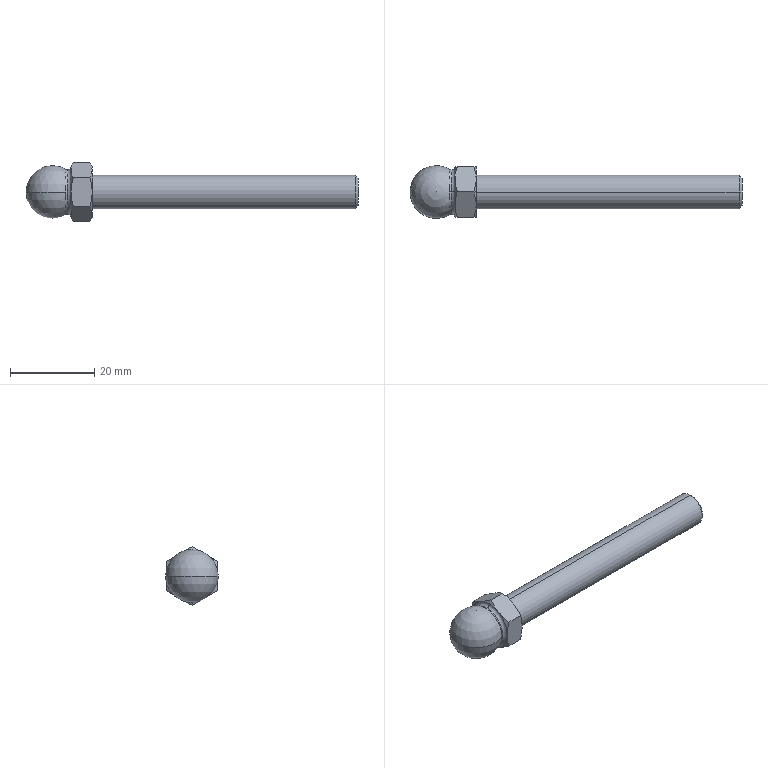Part | STEP file | 343.8-32-M8-63-A | 1 solid | 38 faces | box 78.67 x 12.5 x 13.856 mm | volume 4761 mm3 | cone 16 | plane 14 | torus 4 | sphere 2 | cylinder 2 | commonest cylinder face diameters 8 x2